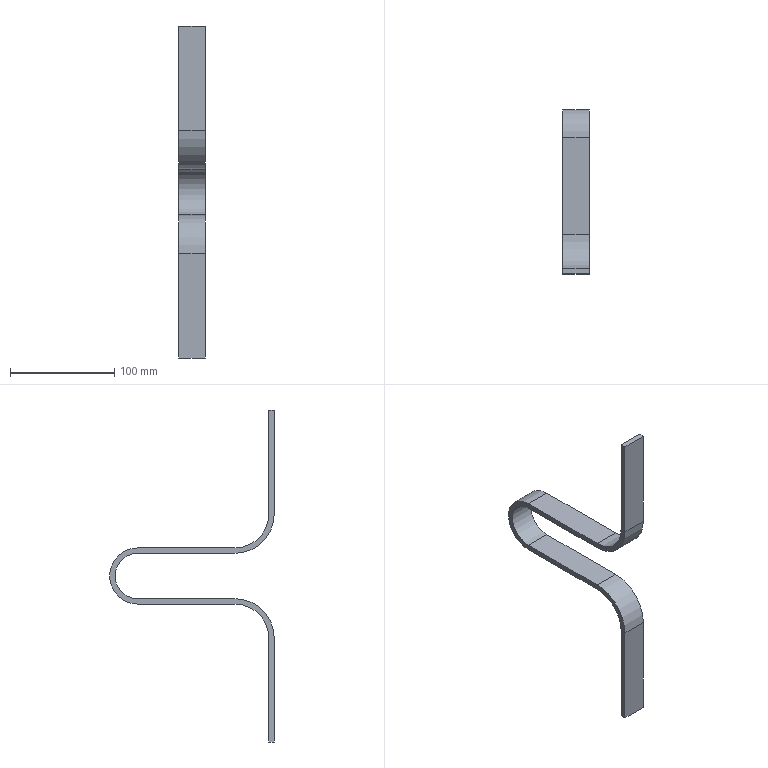Part | STEP file | 0245_Z_103_UM25-8YU-232-SCNUW_2 | 1 solid | 18 faces | box 25 x 158.2 x 319 mm | volume 74610 mm3 | plane 12 | cylinder 6 | commonest cylinder face diameters 65 x2 75.4 x2 43.6 x1 54 x1
STEP:
#1=CARTESIAN_POINT('',(0.,0.,0.));
#2=DIRECTION('',(0.,0.,1.));
#3=DIRECTION('',(1.,0.,0.));
#4=AXIS2_PLACEMENT_3D('',#1,#2,#3);
#5=CARTESIAN_POINT('',(-12.5,5.2,0.));
#6=VERTEX_POINT('',#5);
#7=CARTESIAN_POINT('',(-12.5,0.,0.));
#8=VERTEX_POINT('',#7);
#9=CARTESIAN_POINT('',(-12.5,5.2,0.));
#10=DIRECTION('',(0.,-1.,0.));
#11=VECTOR('',#10,1.);
#12=LINE('',#9,#11);
#13=CARTESIAN_POINT('',(12.5,5.2,0.));
#14=DIRECTION('',(0.,0.,-1.));
#15=DIRECTION('',(-1.,0.,0.));
#16=AXIS2_PLACEMENT_3D('',#13,#14,#15);
#17=PLANE('',#16);
#18=CARTESIAN_POINT('',(25.,0.));
#19=DIRECTION('',(0.,-1.));
#20=VECTOR('',#19,1.);
#21=LINE('',#18,#20);
#22=(GEOMETRIC_REPRESENTATION_CONTEXT(2)PARAMETRIC_REPRESENTATION_CONTEXT()REPRESENTATION_CONTEXT('',''));
#23=DEFINITIONAL_REPRESENTATION('',(#21),#22);
#24=PCURVE('',#17,#23);
#25=CARTESIAN_POINT('',(-12.5,37.7,-100.));
#26=DIRECTION('',(1.,0.,0.));
#27=DIRECTION('',(0.,0.,-1.));
#28=AXIS2_PLACEMENT_3D('',#25,#26,#27);
#29=PLANE('',#28);
#30=CARTESIAN_POINT('',(-100.,-32.5));
#31=DIRECTION('',(0.,-1.));
#32=VECTOR('',#31,1.);
#33=LINE('',#30,#32);
#34=(GEOMETRIC_REPRESENTATION_CONTEXT(2)PARAMETRIC_REPRESENTATION_CONTEXT()REPRESENTATION_CONTEXT('',''));
#35=DEFINITIONAL_REPRESENTATION('',(#33),#34);
#36=PCURVE('',#29,#35);
#37=SURFACE_CURVE('',#12,(#24,#36),.PCURVE_S1.);
#38=EDGE_CURVE('',#6,#8,#37,.T.);
#39=ORIENTED_EDGE('',*,*,#38,.T.);
#40=CARTESIAN_POINT('',(12.5,0.,0.));
#41=VERTEX_POINT('',#40);
#42=CARTESIAN_POINT('',(12.5,0.,0.));
#43=DIRECTION('',(-1.,0.,0.));
#44=VECTOR('',#43,1.);
#45=LINE('',#42,#44);
#46=CARTESIAN_POINT('',(0.,-5.2));
#47=DIRECTION('',(1.,0.));
#48=VECTOR('',#47,1.);
#49=LINE('',#46,#48);
#50=(GEOMETRIC_REPRESENTATION_CONTEXT(2)PARAMETRIC_REPRESENTATION_CONTEXT()REPRESENTATION_CONTEXT('',''));
#51=DEFINITIONAL_REPRESENTATION('',(#49),#50);
#52=PCURVE('',#17,#51);
#53=CARTESIAN_POINT('',(12.5,0.,0.));
#54=DIRECTION('',(0.,1.,0.));
#55=DIRECTION('',(0.,0.,1.));
#56=AXIS2_PLACEMENT_3D('',#53,#54,#55);
#57=PLANE('',#56);
#58=CARTESIAN_POINT('',(0.,0.));
#59=DIRECTION('',(0.,-1.));
#60=VECTOR('',#59,1.);
#61=LINE('',#58,#60);
#62=(GEOMETRIC_REPRESENTATION_CONTEXT(2)PARAMETRIC_REPRESENTATION_CONTEXT()REPRESENTATION_CONTEXT('',''));
#63=DEFINITIONAL_REPRESENTATION('',(#61),#62);
#64=PCURVE('',#57,#63);
#65=SURFACE_CURVE('',#45,(#52,#64),.PCURVE_S1.);
#66=EDGE_CURVE('',#41,#8,#65,.T.);
#67=ORIENTED_EDGE('',*,*,#66,.F.);
#68=CARTESIAN_POINT('',(12.5,5.2,0.));
#69=VERTEX_POINT('',#68);
#70=CARTESIAN_POINT('',(12.5,5.2,0.));
#71=DIRECTION('',(0.,-1.,0.));
#72=VECTOR('',#71,1.);
#73=LINE('',#70,#72);
#74=CARTESIAN_POINT('',(0.,0.));
#75=DIRECTION('',(0.,-1.));
#76=VECTOR('',#75,1.);
#77=LINE('',#74,#76);
#78=(GEOMETRIC_REPRESENTATION_CONTEXT(2)PARAMETRIC_REPRESENTATION_CONTEXT()REPRESENTATION_CONTEXT('',''));
#79=DEFINITIONAL_REPRESENTATION('',(#77),#78);
#80=PCURVE('',#17,#79);
#81=CARTESIAN_POINT('',(12.5,37.7,-100.));
#82=DIRECTION('',(1.,0.,0.));
#83=DIRECTION('',(0.,0.,-1.));
#84=AXIS2_PLACEMENT_3D('',#81,#82,#83);
#85=PLANE('',#84);
#86=CARTESIAN_POINT('',(-100.,-32.5));
#87=DIRECTION('',(0.,-1.));
#88=VECTOR('',#87,1.);
#89=LINE('',#86,#88);
#90=(GEOMETRIC_REPRESENTATION_CONTEXT(2)PARAMETRIC_REPRESENTATION_CONTEXT()REPRESENTATION_CONTEXT('',''));
#91=DEFINITIONAL_REPRESENTATION('',(#89),#90);
#92=PCURVE('',#85,#91);
#93=SURFACE_CURVE('',#73,(#80,#92),.PCURVE_S1.);
#94=EDGE_CURVE('',#69,#41,#93,.T.);
#95=ORIENTED_EDGE('',*,*,#94,.F.);
#96=CARTESIAN_POINT('',(12.5,5.2,0.));
#97=DIRECTION('',(-1.,0.,0.));
#98=VECTOR('',#97,1.);
#99=LINE('',#96,#98);
#100=CARTESIAN_POINT('',(0.,0.));
#101=DIRECTION('',(1.,0.));
#102=VECTOR('',#101,1.);
#103=LINE('',#100,#102);
#104=(GEOMETRIC_REPRESENTATION_CONTEXT(2)PARAMETRIC_REPRESENTATION_CONTEXT()REPRESENTATION_CONTEXT('',''));
#105=DEFINITIONAL_REPRESENTATION('',(#103),#104);
#106=PCURVE('',#17,#105);
#107=CARTESIAN_POINT('',(12.5,5.2,0.));
#108=DIRECTION('',(0.,-1.,0.));
#109=DIRECTION('',(0.,0.,-1.));
#110=AXIS2_PLACEMENT_3D('',#107,#108,#109);
#111=PLANE('',#110);
#112=CARTESIAN_POINT('',(0.,0.));
#113=DIRECTION('',(0.,-1.));
#114=VECTOR('',#113,1.);
#115=LINE('',#112,#114);
#116=(GEOMETRIC_REPRESENTATION_CONTEXT(2)PARAMETRIC_REPRESENTATION_CONTEXT()REPRESENTATION_CONTEXT('',''));
#117=DEFINITIONAL_REPRESENTATION('',(#115),#116);
#118=PCURVE('',#111,#117);
#119=SURFACE_CURVE('',#99,(#106,#118),.PCURVE_S1.);
#120=EDGE_CURVE('',#69,#6,#119,.T.);
#121=ORIENTED_EDGE('',*,*,#120,.T.);
#122=EDGE_LOOP('',(#39,#67,#95,#121));
#123=FACE_BOUND('',#122,.T.);
#124=ADVANCED_FACE('',(#123),#17,.F.);
#125=CARTESIAN_POINT('',(-12.5,0.,-100.));
#126=VERTEX_POINT('',#125);
#127=CARTESIAN_POINT('',(-12.5,0.,0.));
#128=DIRECTION('',(0.,0.,-1.));
#129=VECTOR('',#128,1.);
#130=LINE('',#127,#129);
#131=CARTESIAN_POINT('',(0.,-25.));
#132=DIRECTION('',(-1.,0.));
#133=VECTOR('',#132,1.);
#134=LINE('',#131,#133);
#135=(GEOMETRIC_REPRESENTATION_CONTEXT(2)PARAMETRIC_REPRESENTATION_CONTEXT()REPRESENTATION_CONTEXT('',''));
#136=DEFINITIONAL_REPRESENTATION('',(#134),#135);
#137=PCURVE('',#57,#136);
#138=CARTESIAN_POINT('',(-100.,-37.7));
#139=DIRECTION('',(1.,0.));
#140=VECTOR('',#139,1.);
#141=LINE('',#138,#140);
#142=(GEOMETRIC_REPRESENTATION_CONTEXT(2)PARAMETRIC_REPRESENTATION_CONTEXT()REPRESENTATION_CONTEXT('',''));
#143=DEFINITIONAL_REPRESENTATION('',(#141),#142);
#144=PCURVE('',#29,#143);
#145=SURFACE_CURVE('',#130,(#137,#144),.PCURVE_S1.);
#146=EDGE_CURVE('',#8,#126,#145,.T.);
#147=ORIENTED_EDGE('',*,*,#146,.T.);
#148=CARTESIAN_POINT('',(12.5,0.,-100.));
#149=VERTEX_POINT('',#148);
#150=CARTESIAN_POINT('',(12.5,0.,-100.));
#151=DIRECTION('',(-1.,0.,0.));
#152=VECTOR('',#151,1.);
#153=LINE('',#150,#152);
#154=CARTESIAN_POINT('',(-100.,0.));
#155=DIRECTION('',(0.,-1.));
#156=VECTOR('',#155,1.);
#157=LINE('',#154,#156);
#158=(GEOMETRIC_REPRESENTATION_CONTEXT(2)PARAMETRIC_REPRESENTATION_CONTEXT()REPRESENTATION_CONTEXT('',''));
#159=DEFINITIONAL_REPRESENTATION('',(#157),#158);
#160=PCURVE('',#57,#159);
#161=CARTESIAN_POINT('',(12.5,37.7,-100.));
#162=DIRECTION('',(-1.,0.,0.));
#163=DIRECTION('',(0.,0.,1.));
#164=AXIS2_PLACEMENT_3D('',#161,#162,#163);
#165=CYLINDRICAL_SURFACE('',#164,37.7);
#166=CARTESIAN_POINT('',(4.712,0.));
#167=DIRECTION('',(0.,1.));
#168=VECTOR('',#167,1.);
#169=LINE('',#166,#168);
#170=(GEOMETRIC_REPRESENTATION_CONTEXT(2)PARAMETRIC_REPRESENTATION_CONTEXT()REPRESENTATION_CONTEXT('',''));
#171=DEFINITIONAL_REPRESENTATION('',(#169),#170);
#172=PCURVE('',#165,#171);
#173=SURFACE_CURVE('',#153,(#160,#172),.PCURVE_S1.);
#174=EDGE_CURVE('',#149,#126,#173,.T.);
#175=ORIENTED_EDGE('',*,*,#174,.F.);
#176=CARTESIAN_POINT('',(12.5,0.,0.));
#177=DIRECTION('',(0.,0.,-1.));
#178=VECTOR('',#177,1.);
#179=LINE('',#176,#178);
#180=CARTESIAN_POINT('',(0.,0.));
#181=DIRECTION('',(-1.,0.));
#182=VECTOR('',#181,1.);
#183=LINE('',#180,#182);
#184=(GEOMETRIC_REPRESENTATION_CONTEXT(2)PARAMETRIC_REPRESENTATION_CONTEXT()REPRESENTATION_CONTEXT('',''));
#185=DEFINITIONAL_REPRESENTATION('',(#183),#184);
#186=PCURVE('',#57,#185);
#187=CARTESIAN_POINT('',(-100.,-37.7));
#188=DIRECTION('',(1.,0.));
#189=VECTOR('',#188,1.);
#190=LINE('',#187,#189);
#191=(GEOMETRIC_REPRESENTATION_CONTEXT(2)PARAMETRIC_REPRESENTATION_CONTEXT()REPRESENTATION_CONTEXT('',''));
#192=DEFINITIONAL_REPRESENTATION('',(#190),#191);
#193=PCURVE('',#85,#192);
#194=SURFACE_CURVE('',#179,(#186,#193),.PCURVE_S1.);
#195=EDGE_CURVE('',#41,#149,#194,.T.);
#196=ORIENTED_EDGE('',*,*,#195,.F.);
#197=ORIENTED_EDGE('',*,*,#66,.T.);
#198=EDGE_LOOP('',(#147,#175,#196,#197));
#199=FACE_BOUND('',#198,.T.);
#200=ADVANCED_FACE('',(#199),#57,.F.);
#201=CARTESIAN_POINT('',(-12.5,37.7,-137.7));
#202=VERTEX_POINT('',#201);
#203=CARTESIAN_POINT('',(-12.5,37.7,-100.));
#204=DIRECTION('',(1.,0.,0.));
#205=DIRECTION('',(0.,0.,-1.));
#206=AXIS2_PLACEMENT_3D('',#203,#204,#205);
#207=CIRCLE('',#206,37.7);
#208=CARTESIAN_POINT('',(9.425,25.));
#209=DIRECTION('',(-1.,0.));
#210=VECTOR('',#209,1.);
#211=LINE('',#208,#210);
#212=(GEOMETRIC_REPRESENTATION_CONTEXT(2)PARAMETRIC_REPRESENTATION_CONTEXT()REPRESENTATION_CONTEXT('',''));
#213=DEFINITIONAL_REPRESENTATION('',(#211),#212);
#214=PCURVE('',#165,#213);
#215=CARTESIAN_POINT('',(0.,0.));
#216=DIRECTION('',(1.,0.));
#217=AXIS2_PLACEMENT_2D('',#215,#216);
#218=CIRCLE('',#217,37.7);
#219=(GEOMETRIC_REPRESENTATION_CONTEXT(2)PARAMETRIC_REPRESENTATION_CONTEXT()REPRESENTATION_CONTEXT('',''));
#220=DEFINITIONAL_REPRESENTATION('',(#218),#219);
#221=PCURVE('',#29,#220);
#222=SURFACE_CURVE('',#207,(#214,#221),.PCURVE_S1.);
#223=EDGE_CURVE('',#126,#202,#222,.T.);
#224=ORIENTED_EDGE('',*,*,#223,.T.);
#225=CARTESIAN_POINT('',(12.5,37.7,-137.7));
#226=VERTEX_POINT('',#225);
#227=CARTESIAN_POINT('',(12.5,37.7,-137.7));
#228=DIRECTION('',(-1.,0.,0.));
#229=VECTOR('',#228,1.);
#230=LINE('',#227,#229);
#231=CARTESIAN_POINT('',(3.142,0.));
#232=DIRECTION('',(0.,1.));
#233=VECTOR('',#232,1.);
#234=LINE('',#231,#233);
#235=(GEOMETRIC_REPRESENTATION_CONTEXT(2)PARAMETRIC_REPRESENTATION_CONTEXT()REPRESENTATION_CONTEXT('',''));
#236=DEFINITIONAL_REPRESENTATION('',(#234),#235);
#237=PCURVE('',#165,#236);
#238=CARTESIAN_POINT('',(12.5,37.7,-137.7));
#239=DIRECTION('',(0.,0.,1.));
#240=DIRECTION('',(0.,-1.,0.));
#241=AXIS2_PLACEMENT_3D('',#238,#239,#240);
#242=PLANE('',#241);
#243=CARTESIAN_POINT('',(0.,0.));
#244=DIRECTION('',(0.,-1.));
#245=VECTOR('',#244,1.);
#246=LINE('',#243,#245);
#247=(GEOMETRIC_REPRESENTATION_CONTEXT(2)PARAMETRIC_REPRESENTATION_CONTEXT()REPRESENTATION_CONTEXT('',''));
#248=DEFINITIONAL_REPRESENTATION('',(#246),#247);
#249=PCURVE('',#242,#248);
#250=SURFACE_CURVE('',#230,(#237,#249),.PCURVE_S1.);
#251=EDGE_CURVE('',#226,#202,#250,.T.);
#252=ORIENTED_EDGE('',*,*,#251,.F.);
#253=CARTESIAN_POINT('',(12.5,37.7,-100.));
#254=DIRECTION('',(1.,0.,0.));
#255=DIRECTION('',(0.,0.,-1.));
#256=AXIS2_PLACEMENT_3D('',#253,#254,#255);
#257=CIRCLE('',#256,37.7);
#258=CARTESIAN_POINT('',(9.425,0.));
#259=DIRECTION('',(-1.,0.));
#260=VECTOR('',#259,1.);
#261=LINE('',#258,#260);
#262=(GEOMETRIC_REPRESENTATION_CONTEXT(2)PARAMETRIC_REPRESENTATION_CONTEXT()REPRESENTATION_CONTEXT('',''));
#263=DEFINITIONAL_REPRESENTATION('',(#261),#262);
#264=PCURVE('',#165,#263);
#265=CARTESIAN_POINT('',(0.,0.));
#266=DIRECTION('',(1.,0.));
#267=AXIS2_PLACEMENT_2D('',#265,#266);
#268=CIRCLE('',#267,37.7);
#269=(GEOMETRIC_REPRESENTATION_CONTEXT(2)PARAMETRIC_REPRESENTATION_CONTEXT()REPRESENTATION_CONTEXT('',''));
#270=DEFINITIONAL_REPRESENTATION('',(#268),#269);
#271=PCURVE('',#85,#270);
#272=SURFACE_CURVE('',#257,(#264,#271),.PCURVE_S1.);
#273=EDGE_CURVE('',#149,#226,#272,.T.);
#274=ORIENTED_EDGE('',*,*,#273,.F.);
#275=ORIENTED_EDGE('',*,*,#174,.T.);
#276=EDGE_LOOP('',(#224,#252,#274,#275));
#277=FACE_BOUND('',#276,.T.);
#278=ADVANCED_FACE('',(#277),#165,.T.);
#279=CARTESIAN_POINT('',(-12.5,131.2,-137.7));
#280=VERTEX_POINT('',#279);
#281=CARTESIAN_POINT('',(-12.5,37.7,-137.7));
#282=DIRECTION('',(0.,1.,0.));
#283=VECTOR('',#282,1.);
#284=LINE('',#281,#283);
#285=CARTESIAN_POINT('',(0.,-25.));
#286=DIRECTION('',(-1.,0.));
#287=VECTOR('',#286,1.);
#288=LINE('',#285,#287);
#289=(GEOMETRIC_REPRESENTATION_CONTEXT(2)PARAMETRIC_REPRESENTATION_CONTEXT()REPRESENTATION_CONTEXT('',''));
#290=DEFINITIONAL_REPRESENTATION('',(#288),#289);
#291=PCURVE('',#242,#290);
#292=CARTESIAN_POINT('',(37.7,0.));
#293=DIRECTION('',(0.,1.));
#294=VECTOR('',#293,1.);
#295=LINE('',#292,#294);
#296=(GEOMETRIC_REPRESENTATION_CONTEXT(2)PARAMETRIC_REPRESENTATION_CONTEXT()REPRESENTATION_CONTEXT('',''));
#297=DEFINITIONAL_REPRESENTATION('',(#295),#296);
#298=PCURVE('',#29,#297);
#299=SURFACE_CURVE('',#284,(#291,#298),.PCURVE_S1.);
#300=EDGE_CURVE('',#202,#280,#299,.T.);
#301=ORIENTED_EDGE('',*,*,#300,.T.);
#302=CARTESIAN_POINT('',(12.5,131.2,-137.7));
#303=VERTEX_POINT('',#302);
#304=CARTESIAN_POINT('',(12.5,131.2,-137.7));
#305=DIRECTION('',(-1.,0.,0.));
#306=VECTOR('',#305,1.);
#307=LINE('',#304,#306);
#308=CARTESIAN_POINT('',(-93.5,0.));
#309=DIRECTION('',(0.,-1.));
#310=VECTOR('',#309,1.);
#311=LINE('',#308,#310);
#312=(GEOMETRIC_REPRESENTATION_CONTEXT(2)PARAMETRIC_REPRESENTATION_CONTEXT()REPRESENTATION_CONTEXT('',''));
#313=DEFINITIONAL_REPRESENTATION('',(#311),#312);
#314=PCURVE('',#242,#313);
#315=CARTESIAN_POINT('',(12.5,131.2,-159.5));
#316=DIRECTION('',(-1.,0.,0.));
#317=DIRECTION('',(0.,0.,1.));
#318=AXIS2_PLACEMENT_3D('',#315,#316,#317);
#319=CYLINDRICAL_SURFACE('',#318,21.8);
#320=CARTESIAN_POINT('',(0.,0.));
#321=DIRECTION('',(0.,1.));
#322=VECTOR('',#321,1.);
#323=LINE('',#320,#322);
#324=(GEOMETRIC_REPRESENTATION_CONTEXT(2)PARAMETRIC_REPRESENTATION_CONTEXT()REPRESENTATION_CONTEXT('',''));
#325=DEFINITIONAL_REPRESENTATION('',(#323),#324);
#326=PCURVE('',#319,#325);
#327=SURFACE_CURVE('',#307,(#314,#326),.PCURVE_S1.);
#328=EDGE_CURVE('',#303,#280,#327,.T.);
#329=ORIENTED_EDGE('',*,*,#328,.F.);
#330=CARTESIAN_POINT('',(12.5,37.7,-137.7));
#331=DIRECTION('',(0.,1.,0.));
#332=VECTOR('',#331,1.);
#333=LINE('',#330,#332);
#334=CARTESIAN_POINT('',(0.,0.));
#335=DIRECTION('',(-1.,0.));
#336=VECTOR('',#335,1.);
#337=LINE('',#334,#336);
#338=(GEOMETRIC_REPRESENTATION_CONTEXT(2)PARAMETRIC_REPRESENTATION_CONTEXT()REPRESENTATION_CONTEXT('',''));
#339=DEFINITIONAL_REPRESENTATION('',(#337),#338);
#340=PCURVE('',#242,#339);
#341=CARTESIAN_POINT('',(37.7,0.));
#342=DIRECTION('',(0.,1.));
#343=VECTOR('',#342,1.);
#344=LINE('',#341,#343);
#345=(GEOMETRIC_REPRESENTATION_CONTEXT(2)PARAMETRIC_REPRESENTATION_CONTEXT()REPRESENTATION_CONTEXT('',''));
#346=DEFINITIONAL_REPRESENTATION('',(#344),#345);
#347=PCURVE('',#85,#346);
#348=SURFACE_CURVE('',#333,(#340,#347),.PCURVE_S1.);
#349=EDGE_CURVE('',#226,#303,#348,.T.);
#350=ORIENTED_EDGE('',*,*,#349,.F.);
#351=ORIENTED_EDGE('',*,*,#251,.T.);
#352=EDGE_LOOP('',(#301,#329,#350,#351));
#353=FACE_BOUND('',#352,.T.);
#354=ADVANCED_FACE('',(#353),#242,.F.);
#355=ORIENTED_EDGE('',*,*,#328,.F.);
#356=CARTESIAN_POINT('',(12.5,131.2,-181.3));
#357=VERTEX_POINT('',#356);
#358=CARTESIAN_POINT('',(12.5,131.2,-159.5));
#359=DIRECTION('',(-1.,0.,0.));
#360=DIRECTION('',(0.,0.,1.));
#361=AXIS2_PLACEMENT_3D('',#358,#359,#360);
#362=CIRCLE('',#361,21.8);
#363=CARTESIAN_POINT('',(0.,0.));
#364=DIRECTION('',(1.,0.));
#365=VECTOR('',#364,1.);
#366=LINE('',#363,#365);
#367=(GEOMETRIC_REPRESENTATION_CONTEXT(2)PARAMETRIC_REPRESENTATION_CONTEXT()REPRESENTATION_CONTEXT('',''));
#368=DEFINITIONAL_REPRESENTATION('',(#366),#367);
#369=PCURVE('',#319,#368);
#370=CARTESIAN_POINT('',(37.7,93.5));
#371=CARTESIAN_POINT('',(37.7,131.259));
#372=CARTESIAN_POINT('',(70.4,112.379));
#373=CARTESIAN_POINT('',(103.1,93.5));
#374=CARTESIAN_POINT('',(70.4,74.621));
#375=CARTESIAN_POINT('',(37.7,55.741));
#376=CARTESIAN_POINT('',(37.7,93.5));
#377=(BOUNDED_CURVE()B_SPLINE_CURVE(2,(#370,#371,#372,#373,#374,#375,#376),.UNSPECIFIED.,.T.,.F.)B_SPLINE_CURVE_WITH_KNOTS((1,2,2,2,2,1),(-2.094,0.,2.094,4.189,6.283,8.378),.UNSPECIFIED.)CURVE()GEOMETRIC_REPRESENTATION_ITEM()RATIONAL_B_SPLINE_CURVE((1.,0.5,1.,0.5,1.,0.5,1.))REPRESENTATION_ITEM(''));
#378=(GEOMETRIC_REPRESENTATION_CONTEXT(2)PARAMETRIC_REPRESENTATION_CONTEXT()REPRESENTATION_CONTEXT('',''));
#379=DEFINITIONAL_REPRESENTATION('',(#377),#378);
#380=PCURVE('',#85,#379);
#381=SURFACE_CURVE('',#362,(#369,#380),.PCURVE_S1.);
#382=EDGE_CURVE('',#303,#357,#381,.T.);
#383=ORIENTED_EDGE('',*,*,#382,.T.);
#384=CARTESIAN_POINT('',(-12.5,131.2,-181.3));
#385=VERTEX_POINT('',#384);
#386=CARTESIAN_POINT('',(12.5,131.2,-181.3));
#387=DIRECTION('',(-1.,0.,0.));
#388=VECTOR('',#387,1.);
#389=LINE('',#386,#388);
#390=CARTESIAN_POINT('',(3.142,0.));
#391=DIRECTION('',(0.,1.));
#392=VECTOR('',#391,1.);
#393=LINE('',#390,#392);
#394=(GEOMETRIC_REPRESENTATION_CONTEXT(2)PARAMETRIC_REPRESENTATION_CONTEXT()REPRESENTATION_CONTEXT('',''));
#395=DEFINITIONAL_REPRESENTATION('',(#393),#394);
#396=PCURVE('',#319,#395);
#397=CARTESIAN_POINT('',(12.5,131.2,-181.3));
#398=DIRECTION('',(0.,0.,-1.));
#399=DIRECTION('',(0.,1.,0.));
#400=AXIS2_PLACEMENT_3D('',#397,#398,#399);
#401=PLANE('',#400);
#402=CARTESIAN_POINT('',(0.,0.));
#403=DIRECTION('',(0.,-1.));
#404=VECTOR('',#403,1.);
#405=LINE('',#402,#404);
#406=(GEOMETRIC_REPRESENTATION_CONTEXT(2)PARAMETRIC_REPRESENTATION_CONTEXT()REPRESENTATION_CONTEXT('',''));
#407=DEFINITIONAL_REPRESENTATION('',(#405),#406);
#408=PCURVE('',#401,#407);
#409=SURFACE_CURVE('',#389,(#396,#408),.PCURVE_S1.);
#410=EDGE_CURVE('',#357,#385,#409,.T.);
#411=ORIENTED_EDGE('',*,*,#410,.T.);
#412=CARTESIAN_POINT('',(-12.5,131.2,-159.5));
#413=DIRECTION('',(-1.,0.,0.));
#414=DIRECTION('',(0.,0.,1.));
#415=AXIS2_PLACEMENT_3D('',#412,#413,#414);
#416=CIRCLE('',#415,21.8);
#417=CARTESIAN_POINT('',(0.,25.));
#418=DIRECTION('',(1.,0.));
#419=VECTOR('',#418,1.);
#420=LINE('',#417,#419);
#421=(GEOMETRIC_REPRESENTATION_CONTEXT(2)PARAMETRIC_REPRESENTATION_CONTEXT()REPRESENTATION_CONTEXT('',''));
#422=DEFINITIONAL_REPRESENTATION('',(#420),#421);
#423=PCURVE('',#319,#422);
#424=CARTESIAN_POINT('',(37.7,93.5));
#425=CARTESIAN_POINT('',(37.7,131.259));
#426=CARTESIAN_POINT('',(70.4,112.379));
#427=CARTESIAN_POINT('',(103.1,93.5));
#428=CARTESIAN_POINT('',(70.4,74.621));
#429=CARTESIAN_POINT('',(37.7,55.741));
#430=CARTESIAN_POINT('',(37.7,93.5));
#431=(BOUNDED_CURVE()B_SPLINE_CURVE(2,(#424,#425,#426,#427,#428,#429,#430),.UNSPECIFIED.,.T.,.F.)B_SPLINE_CURVE_WITH_KNOTS((1,2,2,2,2,1),(-2.094,0.,2.094,4.189,6.283,8.378),.UNSPECIFIED.)CURVE()GEOMETRIC_REPRESENTATION_ITEM()RATIONAL_B_SPLINE_CURVE((1.,0.5,1.,0.5,1.,0.5,1.))REPRESENTATION_ITEM(''));
#432=(GEOMETRIC_REPRESENTATION_CONTEXT(2)PARAMETRIC_REPRESENTATION_CONTEXT()REPRESENTATION_CONTEXT('',''));
#433=DEFINITIONAL_REPRESENTATION('',(#431),#432);
#434=PCURVE('',#29,#433);
#435=SURFACE_CURVE('',#416,(#423,#434),.PCURVE_S1.);
#436=EDGE_CURVE('',#280,#385,#435,.T.);
#437=ORIENTED_EDGE('',*,*,#436,.F.);
#438=EDGE_LOOP('',(#355,#383,#411,#437));
#439=FACE_BOUND('',#438,.F.);
#440=ADVANCED_FACE('',(#439),#319,.F.);
#441=CARTESIAN_POINT('',(-12.5,37.7,-181.3));
#442=VERTEX_POINT('',#441);
#443=CARTESIAN_POINT('',(-12.5,131.2,-181.3));
#444=DIRECTION('',(0.,-1.,0.));
#445=VECTOR('',#444,1.);
#446=LINE('',#443,#445);
#447=CARTESIAN_POINT('',(0.,-25.));
#448=DIRECTION('',(-1.,0.));
#449=VECTOR('',#448,1.);
#450=LINE('',#447,#449);
#451=(GEOMETRIC_REPRESENTATION_CONTEXT(2)PARAMETRIC_REPRESENTATION_CONTEXT()REPRESENTATION_CONTEXT('',''));
#452=DEFINITIONAL_REPRESENTATION('',(#450),#451);
#453=PCURVE('',#401,#452);
#454=CARTESIAN_POINT('',(81.3,93.5));
#455=DIRECTION('',(0.,-1.));
#456=VECTOR('',#455,1.);
#457=LINE('',#454,#456);
#458=(GEOMETRIC_REPRESENTATION_CONTEXT(2)PARAMETRIC_REPRESENTATION_CONTEXT()REPRESENTATION_CONTEXT('',''));
#459=DEFINITIONAL_REPRESENTATION('',(#457),#458);
#460=PCURVE('',#29,#459);
#461=SURFACE_CURVE('',#446,(#453,#460),.PCURVE_S1.);
#462=EDGE_CURVE('',#385,#442,#461,.T.);
#463=ORIENTED_EDGE('',*,*,#462,.T.);
#464=CARTESIAN_POINT('',(12.5,37.7,-181.3));
#465=VERTEX_POINT('',#464);
#466=CARTESIAN_POINT('',(12.5,37.7,-181.3));
#467=DIRECTION('',(-1.,0.,0.));
#468=VECTOR('',#467,1.);
#469=LINE('',#466,#468);
#470=CARTESIAN_POINT('',(-93.5,0.));
#471=DIRECTION('',(0.,-1.));
#472=VECTOR('',#471,1.);
#473=LINE('',#470,#472);
#474=(GEOMETRIC_REPRESENTATION_CONTEXT(2)PARAMETRIC_REPRESENTATION_CONTEXT()REPRESENTATION_CONTEXT('',''));
#475=DEFINITIONAL_REPRESENTATION('',(#473),#474);
#476=PCURVE('',#401,#475);
#477=CARTESIAN_POINT('',(12.5,37.7,-219.));
#478=DIRECTION('',(-1.,0.,0.));
#479=DIRECTION('',(0.,0.,1.));
#480=AXIS2_PLACEMENT_3D('',#477,#478,#479);
#481=CYLINDRICAL_SURFACE('',#480,37.7);
#482=CARTESIAN_POINT('',(6.283,0.));
#483=DIRECTION('',(0.,1.));
#484=VECTOR('',#483,1.);
#485=LINE('',#482,#484);
#486=(GEOMETRIC_REPRESENTATION_CONTEXT(2)PARAMETRIC_REPRESENTATION_CONTEXT()REPRESENTATION_CONTEXT('',''));
#487=DEFINITIONAL_REPRESENTATION('',(#485),#486);
#488=PCURVE('',#481,#487);
#489=SURFACE_CURVE('',#469,(#476,#488),.PCURVE_S1.);
#490=EDGE_CURVE('',#465,#442,#489,.T.);
#491=ORIENTED_EDGE('',*,*,#490,.F.);
#492=CARTESIAN_POINT('',(12.5,131.2,-181.3));
#493=DIRECTION('',(0.,-1.,0.));
#494=VECTOR('',#493,1.);
#495=LINE('',#492,#494);
#496=CARTESIAN_POINT('',(0.,0.));
#497=DIRECTION('',(-1.,0.));
#498=VECTOR('',#497,1.);
#499=LINE('',#496,#498);
#500=(GEOMETRIC_REPRESENTATION_CONTEXT(2)PARAMETRIC_REPRESENTATION_CONTEXT()REPRESENTATION_CONTEXT('',''));
#501=DEFINITIONAL_REPRESENTATION('',(#499),#500);
#502=PCURVE('',#401,#501);
#503=CARTESIAN_POINT('',(81.3,93.5));
#504=DIRECTION('',(0.,-1.));
#505=VECTOR('',#504,1.);
#506=LINE('',#503,#505);
#507=(GEOMETRIC_REPRESENTATION_CONTEXT(2)PARAMETRIC_REPRESENTATION_CONTEXT()REPRESENTATION_CONTEXT('',''));
#508=DEFINITIONAL_REPRESENTATION('',(#506),#507);
#509=PCURVE('',#85,#508);
#510=SURFACE_CURVE('',#495,(#502,#509),.PCURVE_S1.);
#511=EDGE_CURVE('',#357,#465,#510,.T.);
#512=ORIENTED_EDGE('',*,*,#511,.F.);
#513=ORIENTED_EDGE('',*,*,#410,.T.);
#514=EDGE_LOOP('',(#463,#491,#512,#513));
#515=FACE_BOUND('',#514,.T.);
#516=ADVANCED_FACE('',(#515),#401,.F.);
#517=CARTESIAN_POINT('',(-12.5,0.,-219.));
#518=VERTEX_POINT('',#517);
#519=CARTESIAN_POINT('',(-12.5,37.7,-219.));
#520=DIRECTION('',(1.,0.,0.));
#521=DIRECTION('',(0.,0.,-1.));
#522=AXIS2_PLACEMENT_3D('',#519,#520,#521);
#523=CIRCLE('',#522,37.7);
#524=CARTESIAN_POINT('',(9.425,25.));
#525=DIRECTION('',(-1.,0.));
#526=VECTOR('',#525,1.);
#527=LINE('',#524,#526);
#528=(GEOMETRIC_REPRESENTATION_CONTEXT(2)PARAMETRIC_REPRESENTATION_CONTEXT()REPRESENTATION_CONTEXT('',''));
#529=DEFINITIONAL_REPRESENTATION('',(#527),#528);
#530=PCURVE('',#481,#529);
#531=CARTESIAN_POINT('',(119.,0.));
#532=DIRECTION('',(1.,0.));
#533=AXIS2_PLACEMENT_2D('',#531,#532);
#534=CIRCLE('',#533,37.7);
#535=(GEOMETRIC_REPRESENTATION_CONTEXT(2)PARAMETRIC_REPRESENTATION_CONTEXT()REPRESENTATION_CONTEXT('',''));
#536=DEFINITIONAL_REPRESENTATION('',(#534),#535);
#537=PCURVE('',#29,#536);
#538=SURFACE_CURVE('',#523,(#530,#537),.PCURVE_S1.);
#539=EDGE_CURVE('',#442,#518,#538,.T.);
#540=ORIENTED_EDGE('',*,*,#539,.T.);
#541=CARTESIAN_POINT('',(12.5,0.,-219.));
#542=VERTEX_POINT('',#541);
#543=CARTESIAN_POINT('',(12.5,0.,-219.));
#544=DIRECTION('',(-1.,0.,0.));
#545=VECTOR('',#544,1.);
#546=LINE('',#543,#545);
#547=CARTESIAN_POINT('',(4.712,0.));
#548=DIRECTION('',(0.,1.));
#549=VECTOR('',#548,1.);
#550=LINE('',#547,#549);
#551=(GEOMETRIC_REPRESENTATION_CONTEXT(2)PARAMETRIC_REPRESENTATION_CONTEXT()REPRESENTATION_CONTEXT('',''));
#552=DEFINITIONAL_REPRESENTATION('',(#550),#551);
#553=PCURVE('',#481,#552);
#554=CARTESIAN_POINT('',(12.5,0.,-219.));
#555=DIRECTION('',(0.,1.,0.));
#556=DIRECTION('',(0.,0.,1.));
#557=AXIS2_PLACEMENT_3D('',#554,#555,#556);
#558=PLANE('',#557);
#559=CARTESIAN_POINT('',(0.,0.));
#560=DIRECTION('',(0.,-1.));
#561=VECTOR('',#560,1.);
#562=LINE('',#559,#561);
#563=(GEOMETRIC_REPRESENTATION_CONTEXT(2)PARAMETRIC_REPRESENTATION_CONTEXT()REPRESENTATION_CONTEXT('',''));
#564=DEFINITIONAL_REPRESENTATION('',(#562),#563);
#565=PCURVE('',#558,#564);
#566=SURFACE_CURVE('',#546,(#553,#565),.PCURVE_S1.);
#567=EDGE_CURVE('',#542,#518,#566,.T.);
#568=ORIENTED_EDGE('',*,*,#567,.F.);
#569=CARTESIAN_POINT('',(12.5,37.7,-219.));
#570=DIRECTION('',(1.,0.,0.));
#571=DIRECTION('',(0.,0.,-1.));
#572=AXIS2_PLACEMENT_3D('',#569,#570,#571);
#573=CIRCLE('',#572,37.7);
#574=CARTESIAN_POINT('',(9.425,0.));
#575=DIRECTION('',(-1.,0.));
#576=VECTOR('',#575,1.);
#577=LINE('',#574,#576);
#578=(GEOMETRIC_REPRESENTATION_CONTEXT(2)PARAMETRIC_REPRESENTATION_CONTEXT()REPRESENTATION_CONTEXT('',''));
#579=DEFINITIONAL_REPRESENTATION('',(#577),#578);
#580=PCURVE('',#481,#579);
#581=CARTESIAN_POINT('',(119.,0.));
#582=DIRECTION('',(1.,0.));
#583=AXIS2_PLACEMENT_2D('',#581,#582);
#584=CIRCLE('',#583,37.7);
#585=(GEOMETRIC_REPRESENTATION_CONTEXT(2)PARAMETRIC_REPRESENTATION_CONTEXT()REPRESENTATION_CONTEXT('',''));
#586=DEFINITIONAL_REPRESENTATION('',(#584),#585);
#587=PCURVE('',#85,#586);
#588=SURFACE_CURVE('',#573,(#580,#587),.PCURVE_S1.);
#589=EDGE_CURVE('',#465,#542,#588,.T.);
#590=ORIENTED_EDGE('',*,*,#589,.F.);
#591=ORIENTED_EDGE('',*,*,#490,.T.);
#592=EDGE_LOOP('',(#540,#568,#590,#591));
#593=FACE_BOUND('',#592,.T.);
#594=ADVANCED_FACE('',(#593),#481,.T.);
#595=CARTESIAN_POINT('',(-12.5,0.,-319.));
#596=VERTEX_POINT('',#595);
#597=CARTESIAN_POINT('',(-12.5,0.,-219.));
#598=DIRECTION('',(0.,0.,-1.));
#599=VECTOR('',#598,1.);
#600=LINE('',#597,#599);
#601=CARTESIAN_POINT('',(0.,-25.));
#602=DIRECTION('',(-1.,0.));
#603=VECTOR('',#602,1.);
#604=LINE('',#601,#603);
#605=(GEOMETRIC_REPRESENTATION_CONTEXT(2)PARAMETRIC_REPRESENTATION_CONTEXT()REPRESENTATION_CONTEXT('',''));
#606=DEFINITIONAL_REPRESENTATION('',(#604),#605);
#607=PCURVE('',#558,#606);
#608=CARTESIAN_POINT('',(119.,-37.7));
#609=DIRECTION('',(1.,0.));
#610=VECTOR('',#609,1.);
#611=LINE('',#608,#610);
#612=(GEOMETRIC_REPRESENTATION_CONTEXT(2)PARAMETRIC_REPRESENTATION_CONTEXT()REPRESENTATION_CONTEXT('',''));
#613=DEFINITIONAL_REPRESENTATION('',(#611),#612);
#614=PCURVE('',#29,#613);
#615=SURFACE_CURVE('',#600,(#607,#614),.PCURVE_S1.);
#616=EDGE_CURVE('',#518,#596,#615,.T.);
#617=ORIENTED_EDGE('',*,*,#616,.T.);
#618=CARTESIAN_POINT('',(12.5,0.,-319.));
#619=VERTEX_POINT('',#618);
#620=CARTESIAN_POINT('',(12.5,0.,-319.));
#621=DIRECTION('',(-1.,0.,0.));
#622=VECTOR('',#621,1.);
#623=LINE('',#620,#622);
#624=CARTESIAN_POINT('',(-100.,0.));
#625=DIRECTION('',(0.,-1.));
#626=VECTOR('',#625,1.);
#627=LINE('',#624,#626);
#628=(GEOMETRIC_REPRESENTATION_CONTEXT(2)PARAMETRIC_REPRESENTATION_CONTEXT()REPRESENTATION_CONTEXT('',''));
#629=DEFINITIONAL_REPRESENTATION('',(#627),#628);
#630=PCURVE('',#558,#629);
#631=CARTESIAN_POINT('',(12.5,0.,-319.));
#632=DIRECTION('',(0.,0.,1.));
#633=DIRECTION('',(1.,0.,0.));
#634=AXIS2_PLACEMENT_3D('',#631,#632,#633);
#635=PLANE('',#634);
#636=CARTESIAN_POINT('',(0.,0.));
#637=DIRECTION('',(-1.,0.));
#638=VECTOR('',#637,1.);
#639=LINE('',#636,#638);
#640=(GEOMETRIC_REPRESENTATION_CONTEXT(2)PARAMETRIC_REPRESENTATION_CONTEXT()REPRESENTATION_CONTEXT('',''));
#641=DEFINITIONAL_REPRESENTATION('',(#639),#640);
#642=PCURVE('',#635,#641);
#643=SURFACE_CURVE('',#623,(#630,#642),.PCURVE_S1.);
#644=EDGE_CURVE('',#619,#596,#643,.T.);
#645=ORIENTED_EDGE('',*,*,#644,.F.);
#646=CARTESIAN_POINT('',(12.5,0.,-219.));
#647=DIRECTION('',(0.,0.,-1.));
#648=VECTOR('',#647,1.);
#649=LINE('',#646,#648);
#650=CARTESIAN_POINT('',(0.,0.));
#651=DIRECTION('',(-1.,0.));
#652=VECTOR('',#651,1.);
#653=LINE('',#650,#652);
#654=(GEOMETRIC_REPRESENTATION_CONTEXT(2)PARAMETRIC_REPRESENTATION_CONTEXT()REPRESENTATION_CONTEXT('',''));
#655=DEFINITIONAL_REPRESENTATION('',(#653),#654);
#656=PCURVE('',#558,#655);
#657=CARTESIAN_POINT('',(119.,-37.7));
#658=DIRECTION('',(1.,0.));
#659=VECTOR('',#658,1.);
#660=LINE('',#657,#659);
#661=(GEOMETRIC_REPRESENTATION_CONTEXT(2)PARAMETRIC_REPRESENTATION_CONTEXT()REPRESENTATION_CONTEXT('',''));
#662=DEFINITIONAL_REPRESENTATION('',(#660),#661);
#663=PCURVE('',#85,#662);
#664=SURFACE_CURVE('',#649,(#656,#663),.PCURVE_S1.);
#665=EDGE_CURVE('',#542,#619,#664,.T.);
#666=ORIENTED_EDGE('',*,*,#665,.F.);
#667=ORIENTED_EDGE('',*,*,#567,.T.);
#668=EDGE_LOOP('',(#617,#645,#666,#667));
#669=FACE_BOUND('',#668,.T.);
#670=ADVANCED_FACE('',(#669),#558,.F.);
#671=CARTESIAN_POINT('',(-12.5,5.2,-319.));
#672=VERTEX_POINT('',#671);
#673=CARTESIAN_POINT('',(-12.5,0.,-319.));
#674=DIRECTION('',(0.,1.,0.));
#675=VECTOR('',#674,1.);
#676=LINE('',#673,#675);
#677=CARTESIAN_POINT('',(-25.,0.));
#678=DIRECTION('',(0.,1.));
#679=VECTOR('',#678,1.);
#680=LINE('',#677,#679);
#681=(GEOMETRIC_REPRESENTATION_CONTEXT(2)PARAMETRIC_REPRESENTATION_CONTEXT()REPRESENTATION_CONTEXT('',''));
#682=DEFINITIONAL_REPRESENTATION('',(#680),#681);
#683=PCURVE('',#635,#682);
#684=CARTESIAN_POINT('',(219.,-37.7));
#685=DIRECTION('',(0.,1.));
#686=VECTOR('',#685,1.);
#687=LINE('',#684,#686);
#688=(GEOMETRIC_REPRESENTATION_CONTEXT(2)PARAMETRIC_REPRESENTATION_CONTEXT()REPRESENTATION_CONTEXT('',''));
#689=DEFINITIONAL_REPRESENTATION('',(#687),#688);
#690=PCURVE('',#29,#689);
#691=SURFACE_CURVE('',#676,(#683,#690),.PCURVE_S1.);
#692=EDGE_CURVE('',#596,#672,#691,.T.);
#693=ORIENTED_EDGE('',*,*,#692,.T.);
#694=CARTESIAN_POINT('',(12.5,5.2,-319.));
#695=VERTEX_POINT('',#694);
#696=CARTESIAN_POINT('',(12.5,5.2,-319.));
#697=DIRECTION('',(-1.,0.,0.));
#698=VECTOR('',#697,1.);
#699=LINE('',#696,#698);
#700=CARTESIAN_POINT('',(0.,5.2));
#701=DIRECTION('',(-1.,0.));
#702=VECTOR('',#701,1.);
#703=LINE('',#700,#702);
#704=(GEOMETRIC_REPRESENTATION_CONTEXT(2)PARAMETRIC_REPRESENTATION_CONTEXT()REPRESENTATION_CONTEXT('',''));
#705=DEFINITIONAL_REPRESENTATION('',(#703),#704);
#706=PCURVE('',#635,#705);
#707=CARTESIAN_POINT('',(12.5,5.2,-219.));
#708=DIRECTION('',(0.,-1.,0.));
#709=DIRECTION('',(0.,0.,-1.));
#710=AXIS2_PLACEMENT_3D('',#707,#708,#709);
#711=PLANE('',#710);
#712=CARTESIAN_POINT('',(100.,0.));
#713=DIRECTION('',(0.,-1.));
#714=VECTOR('',#713,1.);
#715=LINE('',#712,#714);
#716=(GEOMETRIC_REPRESENTATION_CONTEXT(2)PARAMETRIC_REPRESENTATION_CONTEXT()REPRESENTATION_CONTEXT('',''));
#717=DEFINITIONAL_REPRESENTATION('',(#715),#716);
#718=PCURVE('',#711,#717);
#719=SURFACE_CURVE('',#699,(#706,#718),.PCURVE_S1.);
#720=EDGE_CURVE('',#695,#672,#719,.T.);
#721=ORIENTED_EDGE('',*,*,#720,.F.);
#722=CARTESIAN_POINT('',(12.5,0.,-319.));
#723=DIRECTION('',(0.,1.,0.));
#724=VECTOR('',#723,1.);
#725=LINE('',#722,#724);
#726=CARTESIAN_POINT('',(0.,0.));
#727=DIRECTION('',(0.,1.));
#728=VECTOR('',#727,1.);
#729=LINE('',#726,#728);
#730=(GEOMETRIC_REPRESENTATION_CONTEXT(2)PARAMETRIC_REPRESENTATION_CONTEXT()REPRESENTATION_CONTEXT('',''));
#731=DEFINITIONAL_REPRESENTATION('',(#729),#730);
#732=PCURVE('',#635,#731);
#733=CARTESIAN_POINT('',(219.,-37.7));
#734=DIRECTION('',(0.,1.));
#735=VECTOR('',#734,1.);
#736=LINE('',#733,#735);
#737=(GEOMETRIC_REPRESENTATION_CONTEXT(2)PARAMETRIC_REPRESENTATION_CONTEXT()REPRESENTATION_CONTEXT('',''));
#738=DEFINITIONAL_REPRESENTATION('',(#736),#737);
#739=PCURVE('',#85,#738);
#740=SURFACE_CURVE('',#725,(#732,#739),.PCURVE_S1.);
#741=EDGE_CURVE('',#619,#695,#740,.T.);
#742=ORIENTED_EDGE('',*,*,#741,.F.);
#743=ORIENTED_EDGE('',*,*,#644,.T.);
#744=EDGE_LOOP('',(#693,#721,#742,#743));
#745=FACE_BOUND('',#744,.T.);
#746=ADVANCED_FACE('',(#745),#635,.F.);
#747=CARTESIAN_POINT('',(-12.5,5.2,-219.));
#748=VERTEX_POINT('',#747);
#749=CARTESIAN_POINT('',(-12.5,5.2,-219.));
#750=DIRECTION('',(0.,0.,1.));
#751=VECTOR('',#750,1.);
#752=LINE('',#749,#751);
#753=CARTESIAN_POINT('',(0.,-25.));
#754=DIRECTION('',(-1.,0.));
#755=VECTOR('',#754,1.);
#756=LINE('',#753,#755);
#757=(GEOMETRIC_REPRESENTATION_CONTEXT(2)PARAMETRIC_REPRESENTATION_CONTEXT()REPRESENTATION_CONTEXT('',''));
#758=DEFINITIONAL_REPRESENTATION('',(#756),#757);
#759=PCURVE('',#711,#758);
#760=CARTESIAN_POINT('',(119.,-32.5));
#761=DIRECTION('',(-1.,0.));
#762=VECTOR('',#761,1.);
#763=LINE('',#760,#762);
#764=(GEOMETRIC_REPRESENTATION_CONTEXT(2)PARAMETRIC_REPRESENTATION_CONTEXT()REPRESENTATION_CONTEXT('',''));
#765=DEFINITIONAL_REPRESENTATION('',(#763),#764);
#766=PCURVE('',#29,#765);
#767=SURFACE_CURVE('',#752,(#759,#766),.PCURVE_S1.);
#768=EDGE_CURVE('',#672,#748,#767,.T.);
#769=ORIENTED_EDGE('',*,*,#768,.T.);
#770=CARTESIAN_POINT('',(12.5,5.2,-219.));
#771=VERTEX_POINT('',#770);
#772=CARTESIAN_POINT('',(12.5,5.2,-219.));
#773=DIRECTION('',(-1.,0.,0.));
#774=VECTOR('',#773,1.);
#775=LINE('',#772,#774);
#776=CARTESIAN_POINT('',(0.,0.));
#777=DIRECTION('',(0.,-1.));
#778=VECTOR('',#777,1.);
#779=LINE('',#776,#778);
#780=(GEOMETRIC_REPRESENTATION_CONTEXT(2)PARAMETRIC_REPRESENTATION_CONTEXT()REPRESENTATION_CONTEXT('',''));
#781=DEFINITIONAL_REPRESENTATION('',(#779),#780);
#782=PCURVE('',#711,#781);
#783=CARTESIAN_POINT('',(12.5,37.7,-219.));
#784=DIRECTION('',(-1.,0.,0.));
#785=DIRECTION('',(0.,0.,1.));
#786=AXIS2_PLACEMENT_3D('',#783,#784,#785);
#787=CYLINDRICAL_SURFACE('',#786,32.5);
#788=CARTESIAN_POINT('',(4.712,0.));
#789=DIRECTION('',(0.,1.));
#790=VECTOR('',#789,1.);
#791=LINE('',#788,#790);
#792=(GEOMETRIC_REPRESENTATION_CONTEXT(2)PARAMETRIC_REPRESENTATION_CONTEXT()REPRESENTATION_CONTEXT('',''));
#793=DEFINITIONAL_REPRESENTATION('',(#791),#792);
#794=PCURVE('',#787,#793);
#795=SURFACE_CURVE('',#775,(#782,#794),.PCURVE_S1.);
#796=EDGE_CURVE('',#771,#748,#795,.T.);
#797=ORIENTED_EDGE('',*,*,#796,.F.);
#798=CARTESIAN_POINT('',(12.5,5.2,-219.));
#799=DIRECTION('',(0.,0.,1.));
#800=VECTOR('',#799,1.);
#801=LINE('',#798,#800);
#802=CARTESIAN_POINT('',(0.,0.));
#803=DIRECTION('',(-1.,0.));
#804=VECTOR('',#803,1.);
#805=LINE('',#802,#804);
#806=(GEOMETRIC_REPRESENTATION_CONTEXT(2)PARAMETRIC_REPRESENTATION_CONTEXT()REPRESENTATION_CONTEXT('',''));
#807=DEFINITIONAL_REPRESENTATION('',(#805),#806);
#808=PCURVE('',#711,#807);
#809=CARTESIAN_POINT('',(119.,-32.5));
#810=DIRECTION('',(-1.,0.));
#811=VECTOR('',#810,1.);
#812=LINE('',#809,#811);
#813=(GEOMETRIC_REPRESENTATION_CONTEXT(2)PARAMETRIC_REPRESENTATION_CONTEXT()REPRESENTATION_CONTEXT('',''));
#814=DEFINITIONAL_REPRESENTATION('',(#812),#813);
#815=PCURVE('',#85,#814);
#816=SURFACE_CURVE('',#801,(#808,#815),.PCURVE_S1.);
#817=EDGE_CURVE('',#695,#771,#816,.T.);
#818=ORIENTED_EDGE('',*,*,#817,.F.);
#819=ORIENTED_EDGE('',*,*,#720,.T.);
#820=EDGE_LOOP('',(#769,#797,#818,#819));
#821=FACE_BOUND('',#820,.T.);
#822=ADVANCED_FACE('',(#821),#711,.F.);
#823=ORIENTED_EDGE('',*,*,#796,.F.);
#824=CARTESIAN_POINT('',(12.5,37.7,-186.5));
#825=VERTEX_POINT('',#824);
#826=CARTESIAN_POINT('',(12.5,37.7,-219.));
#827=DIRECTION('',(-1.,0.,0.));
#828=DIRECTION('',(0.,0.,-1.));
#829=AXIS2_PLACEMENT_3D('',#826,#827,#828);
#830=CIRCLE('',#829,32.5);
#831=CARTESIAN_POINT('',(3.142,0.));
#832=DIRECTION('',(1.,0.));
#833=VECTOR('',#832,1.);
#834=LINE('',#831,#833);
#835=(GEOMETRIC_REPRESENTATION_CONTEXT(2)PARAMETRIC_REPRESENTATION_CONTEXT()REPRESENTATION_CONTEXT('',''));
#836=DEFINITIONAL_REPRESENTATION('',(#834),#835);
#837=PCURVE('',#787,#836);
#838=CARTESIAN_POINT('',(151.5,0.));
#839=CARTESIAN_POINT('',(151.5,-56.292));
#840=CARTESIAN_POINT('',(102.75,-28.146));
#841=CARTESIAN_POINT('',(54.,0.));
#842=CARTESIAN_POINT('',(102.75,28.146));
#843=CARTESIAN_POINT('',(151.5,56.292));
#844=CARTESIAN_POINT('',(151.5,0.));
#845=(BOUNDED_CURVE()B_SPLINE_CURVE(2,(#838,#839,#840,#841,#842,#843,#844),.UNSPECIFIED.,.T.,.F.)B_SPLINE_CURVE_WITH_KNOTS((1,2,2,2,2,1),(-2.094,0.,2.094,4.189,6.283,8.378),.UNSPECIFIED.)CURVE()GEOMETRIC_REPRESENTATION_ITEM()RATIONAL_B_SPLINE_CURVE((1.,0.5,1.,0.5,1.,0.5,1.))REPRESENTATION_ITEM(''));
#846=(GEOMETRIC_REPRESENTATION_CONTEXT(2)PARAMETRIC_REPRESENTATION_CONTEXT()REPRESENTATION_CONTEXT('',''));
#847=DEFINITIONAL_REPRESENTATION('',(#845),#846);
#848=PCURVE('',#85,#847);
#849=SURFACE_CURVE('',#830,(#837,#848),.PCURVE_S1.);
#850=EDGE_CURVE('',#771,#825,#849,.T.);
#851=ORIENTED_EDGE('',*,*,#850,.T.);
#852=CARTESIAN_POINT('',(-12.5,37.7,-186.5));
#853=VERTEX_POINT('',#852);
#854=CARTESIAN_POINT('',(12.5,37.7,-186.5));
#855=DIRECTION('',(-1.,0.,0.));
#856=VECTOR('',#855,1.);
#857=LINE('',#854,#856);
#858=CARTESIAN_POINT('',(6.283,0.));
#859=DIRECTION('',(0.,1.));
#860=VECTOR('',#859,1.);
#861=LINE('',#858,#860);
#862=(GEOMETRIC_REPRESENTATION_CONTEXT(2)PARAMETRIC_REPRESENTATION_CONTEXT()REPRESENTATION_CONTEXT('',''));
#863=DEFINITIONAL_REPRESENTATION('',(#861),#862);
#864=PCURVE('',#787,#863);
#865=CARTESIAN_POINT('',(12.5,131.2,-186.5));
#866=DIRECTION('',(0.,0.,1.));
#867=DIRECTION('',(0.,-1.,0.));
#868=AXIS2_PLACEMENT_3D('',#865,#866,#867);
#869=PLANE('',#868);
#870=CARTESIAN_POINT('',(93.5,0.));
#871=DIRECTION('',(0.,-1.));
#872=VECTOR('',#871,1.);
#873=LINE('',#870,#872);
#874=(GEOMETRIC_REPRESENTATION_CONTEXT(2)PARAMETRIC_REPRESENTATION_CONTEXT()REPRESENTATION_CONTEXT('',''));
#875=DEFINITIONAL_REPRESENTATION('',(#873),#874);
#876=PCURVE('',#869,#875);
#877=SURFACE_CURVE('',#857,(#864,#876),.PCURVE_S1.);
#878=EDGE_CURVE('',#825,#853,#877,.T.);
#879=ORIENTED_EDGE('',*,*,#878,.T.);
#880=CARTESIAN_POINT('',(-12.5,37.7,-219.));
#881=DIRECTION('',(-1.,0.,0.));
#882=DIRECTION('',(0.,0.,-1.));
#883=AXIS2_PLACEMENT_3D('',#880,#881,#882);
#884=CIRCLE('',#883,32.5);
#885=CARTESIAN_POINT('',(3.142,25.));
#886=DIRECTION('',(1.,0.));
#887=VECTOR('',#886,1.);
#888=LINE('',#885,#887);
#889=(GEOMETRIC_REPRESENTATION_CONTEXT(2)PARAMETRIC_REPRESENTATION_CONTEXT()REPRESENTATION_CONTEXT('',''));
#890=DEFINITIONAL_REPRESENTATION('',(#888),#889);
#891=PCURVE('',#787,#890);
#892=CARTESIAN_POINT('',(151.5,0.));
#893=CARTESIAN_POINT('',(151.5,-56.292));
#894=CARTESIAN_POINT('',(102.75,-28.146));
#895=CARTESIAN_POINT('',(54.,0.));
#896=CARTESIAN_POINT('',(102.75,28.146));
#897=CARTESIAN_POINT('',(151.5,56.292));
#898=CARTESIAN_POINT('',(151.5,0.));
#899=(BOUNDED_CURVE()B_SPLINE_CURVE(2,(#892,#893,#894,#895,#896,#897,#898),.UNSPECIFIED.,.T.,.F.)B_SPLINE_CURVE_WITH_KNOTS((1,2,2,2,2,1),(-2.094,0.,2.094,4.189,6.283,8.378),.UNSPECIFIED.)CURVE()GEOMETRIC_REPRESENTATION_ITEM()RATIONAL_B_SPLINE_CURVE((1.,0.5,1.,0.5,1.,0.5,1.))REPRESENTATION_ITEM(''));
#900=(GEOMETRIC_REPRESENTATION_CONTEXT(2)PARAMETRIC_REPRESENTATION_CONTEXT()REPRESENTATION_CONTEXT('',''));
#901=DEFINITIONAL_REPRESENTATION('',(#899),#900);
#902=PCURVE('',#29,#901);
#903=SURFACE_CURVE('',#884,(#891,#902),.PCURVE_S1.);
#904=EDGE_CURVE('',#748,#853,#903,.T.);
#905=ORIENTED_EDGE('',*,*,#904,.F.);
#906=EDGE_LOOP('',(#823,#851,#879,#905));
#907=FACE_BOUND('',#906,.F.);
#908=ADVANCED_FACE('',(#907),#787,.F.);
#909=CARTESIAN_POINT('',(-12.5,131.2,-186.5));
#910=VERTEX_POINT('',#909);
#911=CARTESIAN_POINT('',(-12.5,131.2,-186.5));
#912=DIRECTION('',(0.,1.,0.));
#913=VECTOR('',#912,1.);
#914=LINE('',#911,#913);
#915=CARTESIAN_POINT('',(0.,-25.));
#916=DIRECTION('',(-1.,0.));
#917=VECTOR('',#916,1.);
#918=LINE('',#915,#917);
#919=(GEOMETRIC_REPRESENTATION_CONTEXT(2)PARAMETRIC_REPRESENTATION_CONTEXT()REPRESENTATION_CONTEXT('',''));
#920=DEFINITIONAL_REPRESENTATION('',(#918),#919);
#921=PCURVE('',#869,#920);
#922=CARTESIAN_POINT('',(86.5,93.5));
#923=DIRECTION('',(0.,1.));
#924=VECTOR('',#923,1.);
#925=LINE('',#922,#924);
#926=(GEOMETRIC_REPRESENTATION_CONTEXT(2)PARAMETRIC_REPRESENTATION_CONTEXT()REPRESENTATION_CONTEXT('',''));
#927=DEFINITIONAL_REPRESENTATION('',(#925),#926);
#928=PCURVE('',#29,#927);
#929=SURFACE_CURVE('',#914,(#921,#928),.PCURVE_S1.);
#930=EDGE_CURVE('',#853,#910,#929,.T.);
#931=ORIENTED_EDGE('',*,*,#930,.T.);
#932=CARTESIAN_POINT('',(12.5,131.2,-186.5));
#933=VERTEX_POINT('',#932);
#934=CARTESIAN_POINT('',(12.5,131.2,-186.5));
#935=DIRECTION('',(-1.,0.,0.));
#936=VECTOR('',#935,1.);
#937=LINE('',#934,#936);
#938=CARTESIAN_POINT('',(0.,0.));
#939=DIRECTION('',(0.,-1.));
#940=VECTOR('',#939,1.);
#941=LINE('',#938,#940);
#942=(GEOMETRIC_REPRESENTATION_CONTEXT(2)PARAMETRIC_REPRESENTATION_CONTEXT()REPRESENTATION_CONTEXT('',''));
#943=DEFINITIONAL_REPRESENTATION('',(#941),#942);
#944=PCURVE('',#869,#943);
#945=CARTESIAN_POINT('',(12.5,131.2,-159.5));
#946=DIRECTION('',(-1.,0.,0.));
#947=DIRECTION('',(0.,0.,1.));
#948=AXIS2_PLACEMENT_3D('',#945,#946,#947);
#949=CYLINDRICAL_SURFACE('',#948,27.);
#950=CARTESIAN_POINT('',(3.142,0.));
#951=DIRECTION('',(0.,1.));
#952=VECTOR('',#951,1.);
#953=LINE('',#950,#952);
#954=(GEOMETRIC_REPRESENTATION_CONTEXT(2)PARAMETRIC_REPRESENTATION_CONTEXT()REPRESENTATION_CONTEXT('',''));
#955=DEFINITIONAL_REPRESENTATION('',(#953),#954);
#956=PCURVE('',#949,#955);
#957=SURFACE_CURVE('',#937,(#944,#956),.PCURVE_S1.);
#958=EDGE_CURVE('',#933,#910,#957,.T.);
#959=ORIENTED_EDGE('',*,*,#958,.F.);
#960=CARTESIAN_POINT('',(12.5,131.2,-186.5));
#961=DIRECTION('',(0.,1.,0.));
#962=VECTOR('',#961,1.);
#963=LINE('',#960,#962);
#964=CARTESIAN_POINT('',(0.,0.));
#965=DIRECTION('',(-1.,0.));
#966=VECTOR('',#965,1.);
#967=LINE('',#964,#966);
#968=(GEOMETRIC_REPRESENTATION_CONTEXT(2)PARAMETRIC_REPRESENTATION_CONTEXT()REPRESENTATION_CONTEXT('',''));
#969=DEFINITIONAL_REPRESENTATION('',(#967),#968);
#970=PCURVE('',#869,#969);
#971=CARTESIAN_POINT('',(86.5,93.5));
#972=DIRECTION('',(0.,1.));
#973=VECTOR('',#972,1.);
#974=LINE('',#971,#973);
#975=(GEOMETRIC_REPRESENTATION_CONTEXT(2)PARAMETRIC_REPRESENTATION_CONTEXT()REPRESENTATION_CONTEXT('',''));
#976=DEFINITIONAL_REPRESENTATION('',(#974),#975);
#977=PCURVE('',#85,#976);
#978=SURFACE_CURVE('',#963,(#970,#977),.PCURVE_S1.);
#979=EDGE_CURVE('',#825,#933,#978,.T.);
#980=ORIENTED_EDGE('',*,*,#979,.F.);
#981=ORIENTED_EDGE('',*,*,#878,.T.);
#982=EDGE_LOOP('',(#931,#959,#980,#981));
#983=FACE_BOUND('',#982,.T.);
#984=ADVANCED_FACE('',(#983),#869,.F.);
#985=CARTESIAN_POINT('',(-12.5,131.2,-132.5));
#986=VERTEX_POINT('',#985);
#987=CARTESIAN_POINT('',(-12.5,131.2,-159.5));
#988=DIRECTION('',(1.,0.,0.));
#989=DIRECTION('',(0.,0.,1.));
#990=AXIS2_PLACEMENT_3D('',#987,#988,#989);
#991=CIRCLE('',#990,27.);
#992=CARTESIAN_POINT('',(6.283,25.));
#993=DIRECTION('',(-1.,0.));
#994=VECTOR('',#993,1.);
#995=LINE('',#992,#994);
#996=(GEOMETRIC_REPRESENTATION_CONTEXT(2)PARAMETRIC_REPRESENTATION_CONTEXT()REPRESENTATION_CONTEXT('',''));
#997=DEFINITIONAL_REPRESENTATION('',(#995),#996);
#998=PCURVE('',#949,#997);
#999=CARTESIAN_POINT('',(59.5,93.5));
#1000=DIRECTION('',(-1.,0.));
#1001=AXIS2_PLACEMENT_2D('',#999,#1000);
#1002=CIRCLE('',#1001,27.);
#1003=(GEOMETRIC_REPRESENTATION_CONTEXT(2)PARAMETRIC_REPRESENTATION_CONTEXT()REPRESENTATION_CONTEXT('',''));
#1004=DEFINITIONAL_REPRESENTATION('',(#1002),#1003);
#1005=PCURVE('',#29,#1004);
#1006=SURFACE_CURVE('',#991,(#998,#1005),.PCURVE_S1.);
#1007=EDGE_CURVE('',#910,#986,#1006,.T.);
#1008=ORIENTED_EDGE('',*,*,#1007,.T.);
#1009=CARTESIAN_POINT('',(12.5,131.2,-132.5));
#1010=VERTEX_POINT('',#1009);
#1011=CARTESIAN_POINT('',(12.5,131.2,-132.5));
#1012=DIRECTION('',(-1.,0.,0.));
#1013=VECTOR('',#1012,1.);
#1014=LINE('',#1011,#1013);
#1015=CARTESIAN_POINT('',(0.,0.));
#1016=DIRECTION('',(0.,1.));
#1017=VECTOR('',#1016,1.);
#1018=LINE('',#1015,#1017);
#1019=(GEOMETRIC_REPRESENTATION_CONTEXT(2)PARAMETRIC_REPRESENTATION_CONTEXT()REPRESENTATION_CONTEXT('',''));
#1020=DEFINITIONAL_REPRESENTATION('',(#1018),#1019);
#1021=PCURVE('',#949,#1020);
#1022=CARTESIAN_POINT('',(12.5,37.7,-132.5));
#1023=DIRECTION('',(0.,0.,-1.));
#1024=DIRECTION('',(-1.,0.,0.));
#1025=AXIS2_PLACEMENT_3D('',#1022,#1023,#1024);
#1026=PLANE('',#1025);
#1027=CARTESIAN_POINT('',(0.,93.5));
#1028=DIRECTION('',(1.,0.));
#1029=VECTOR('',#1028,1.);
#1030=LINE('',#1027,#1029);
#1031=(GEOMETRIC_REPRESENTATION_CONTEXT(2)PARAMETRIC_REPRESENTATION_CONTEXT()REPRESENTATION_CONTEXT('',''));
#1032=DEFINITIONAL_REPRESENTATION('',(#1030),#1031);
#1033=PCURVE('',#1026,#1032);
#1034=SURFACE_CURVE('',#1014,(#1021,#1033),.PCURVE_S1.);
#1035=EDGE_CURVE('',#1010,#986,#1034,.T.);
#1036=ORIENTED_EDGE('',*,*,#1035,.F.);
#1037=CARTESIAN_POINT('',(12.5,131.2,-159.5));
#1038=DIRECTION('',(1.,0.,0.));
#1039=DIRECTION('',(0.,0.,1.));
#1040=AXIS2_PLACEMENT_3D('',#1037,#1038,#1039);
#1041=CIRCLE('',#1040,27.);
#1042=CARTESIAN_POINT('',(6.283,0.));
#1043=DIRECTION('',(-1.,0.));
#1044=VECTOR('',#1043,1.);
#1045=LINE('',#1042,#1044);
#1046=(GEOMETRIC_REPRESENTATION_CONTEXT(2)PARAMETRIC_REPRESENTATION_CONTEXT()REPRESENTATION_CONTEXT('',''));
#1047=DEFINITIONAL_REPRESENTATION('',(#1045),#1046);
#1048=PCURVE('',#949,#1047);
#1049=CARTESIAN_POINT('',(59.5,93.5));
#1050=DIRECTION('',(-1.,0.));
#1051=AXIS2_PLACEMENT_2D('',#1049,#1050);
#1052=CIRCLE('',#1051,27.);
#1053=(GEOMETRIC_REPRESENTATION_CONTEXT(2)PARAMETRIC_REPRESENTATION_CONTEXT()REPRESENTATION_CONTEXT('',''));
#1054=DEFINITIONAL_REPRESENTATION('',(#1052),#1053);
#1055=PCURVE('',#85,#1054);
#1056=SURFACE_CURVE('',#1041,(#1048,#1055),.PCURVE_S1.);
#1057=EDGE_CURVE('',#933,#1010,#1056,.T.);
#1058=ORIENTED_EDGE('',*,*,#1057,.F.);
#1059=ORIENTED_EDGE('',*,*,#958,.T.);
#1060=EDGE_LOOP('',(#1008,#1036,#1058,#1059));
#1061=FACE_BOUND('',#1060,.T.);
#1062=ADVANCED_FACE('',(#1061),#949,.T.);
#1063=CARTESIAN_POINT('',(-12.5,37.7,-132.5));
#1064=VERTEX_POINT('',#1063);
#1065=CARTESIAN_POINT('',(-12.5,37.7,-132.5));
#1066=DIRECTION('',(0.,-1.,0.));
#1067=VECTOR('',#1066,1.);
#1068=LINE('',#1065,#1067);
#1069=CARTESIAN_POINT('',(25.,0.));
#1070=DIRECTION('',(0.,-1.));
#1071=VECTOR('',#1070,1.);
#1072=LINE('',#1069,#1071);
#1073=(GEOMETRIC_REPRESENTATION_CONTEXT(2)PARAMETRIC_REPRESENTATION_CONTEXT()REPRESENTATION_CONTEXT('',''));
#1074=DEFINITIONAL_REPRESENTATION('',(#1072),#1073);
#1075=PCURVE('',#1026,#1074);
#1076=CARTESIAN_POINT('',(32.5,0.));
#1077=DIRECTION('',(0.,-1.));
#1078=VECTOR('',#1077,1.);
#1079=LINE('',#1076,#1078);
#1080=(GEOMETRIC_REPRESENTATION_CONTEXT(2)PARAMETRIC_REPRESENTATION_CONTEXT()REPRESENTATION_CONTEXT('',''));
#1081=DEFINITIONAL_REPRESENTATION('',(#1079),#1080);
#1082=PCURVE('',#29,#1081);
#1083=SURFACE_CURVE('',#1068,(#1075,#1082),.PCURVE_S1.);
#1084=EDGE_CURVE('',#986,#1064,#1083,.T.);
#1085=ORIENTED_EDGE('',*,*,#1084,.T.);
#1086=CARTESIAN_POINT('',(12.5,37.7,-132.5));
#1087=VERTEX_POINT('',#1086);
#1088=CARTESIAN_POINT('',(12.5,37.7,-132.5));
#1089=DIRECTION('',(-1.,0.,0.));
#1090=VECTOR('',#1089,1.);
#1091=LINE('',#1088,#1090);
#1092=CARTESIAN_POINT('',(0.,0.));
#1093=DIRECTION('',(1.,0.));
#1094=VECTOR('',#1093,1.);
#1095=LINE('',#1092,#1094);
#1096=(GEOMETRIC_REPRESENTATION_CONTEXT(2)PARAMETRIC_REPRESENTATION_CONTEXT()REPRESENTATION_CONTEXT('',''));
#1097=DEFINITIONAL_REPRESENTATION('',(#1095),#1096);
#1098=PCURVE('',#1026,#1097);
#1099=CARTESIAN_POINT('',(12.5,37.7,-100.));
#1100=DIRECTION('',(-1.,0.,0.));
#1101=DIRECTION('',(0.,0.,1.));
#1102=AXIS2_PLACEMENT_3D('',#1099,#1100,#1101);
#1103=CYLINDRICAL_SURFACE('',#1102,32.5);
#1104=CARTESIAN_POINT('',(3.142,0.));
#1105=DIRECTION('',(0.,1.));
#1106=VECTOR('',#1105,1.);
#1107=LINE('',#1104,#1106);
#1108=(GEOMETRIC_REPRESENTATION_CONTEXT(2)PARAMETRIC_REPRESENTATION_CONTEXT()REPRESENTATION_CONTEXT('',''));
#1109=DEFINITIONAL_REPRESENTATION('',(#1107),#1108);
#1110=PCURVE('',#1103,#1109);
#1111=SURFACE_CURVE('',#1091,(#1098,#1110),.PCURVE_S1.);
#1112=EDGE_CURVE('',#1087,#1064,#1111,.T.);
#1113=ORIENTED_EDGE('',*,*,#1112,.F.);
#1114=CARTESIAN_POINT('',(12.5,37.7,-132.5));
#1115=DIRECTION('',(0.,-1.,0.));
#1116=VECTOR('',#1115,1.);
#1117=LINE('',#1114,#1116);
#1118=CARTESIAN_POINT('',(0.,0.));
#1119=DIRECTION('',(0.,-1.));
#1120=VECTOR('',#1119,1.);
#1121=LINE('',#1118,#1120);
#1122=(GEOMETRIC_REPRESENTATION_CONTEXT(2)PARAMETRIC_REPRESENTATION_CONTEXT()REPRESENTATION_CONTEXT('',''));
#1123=DEFINITIONAL_REPRESENTATION('',(#1121),#1122);
#1124=PCURVE('',#1026,#1123);
#1125=CARTESIAN_POINT('',(32.5,0.));
#1126=DIRECTION('',(0.,-1.));
#1127=VECTOR('',#1126,1.);
#1128=LINE('',#1125,#1127);
#1129=(GEOMETRIC_REPRESENTATION_CONTEXT(2)PARAMETRIC_REPRESENTATION_CONTEXT()REPRESENTATION_CONTEXT('',''));
#1130=DEFINITIONAL_REPRESENTATION('',(#1128),#1129);
#1131=PCURVE('',#85,#1130);
#1132=SURFACE_CURVE('',#1117,(#1124,#1131),.PCURVE_S1.);
#1133=EDGE_CURVE('',#1010,#1087,#1132,.T.);
#1134=ORIENTED_EDGE('',*,*,#1133,.F.);
#1135=ORIENTED_EDGE('',*,*,#1035,.T.);
#1136=EDGE_LOOP('',(#1085,#1113,#1134,#1135));
#1137=FACE_BOUND('',#1136,.T.);
#1138=ADVANCED_FACE('',(#1137),#1026,.F.);
#1139=ORIENTED_EDGE('',*,*,#1112,.F.);
#1140=CARTESIAN_POINT('',(12.5,5.2,-100.));
#1141=VERTEX_POINT('',#1140);
#1142=CARTESIAN_POINT('',(12.5,37.7,-100.));
#1143=DIRECTION('',(-1.,0.,0.));
#1144=DIRECTION('',(0.,0.,-1.));
#1145=AXIS2_PLACEMENT_3D('',#1142,#1143,#1144);
#1146=CIRCLE('',#1145,32.5);
#1147=CARTESIAN_POINT('',(3.142,0.));
#1148=DIRECTION('',(1.,0.));
#1149=VECTOR('',#1148,1.);
#1150=LINE('',#1147,#1149);
#1151=(GEOMETRIC_REPRESENTATION_CONTEXT(2)PARAMETRIC_REPRESENTATION_CONTEXT()REPRESENTATION_CONTEXT('',''));
#1152=DEFINITIONAL_REPRESENTATION('',(#1150),#1151);
#1153=PCURVE('',#1103,#1152);
#1154=CARTESIAN_POINT('',(32.5,0.));
#1155=CARTESIAN_POINT('',(32.5,-56.292));
#1156=CARTESIAN_POINT('',(-16.25,-28.146));
#1157=CARTESIAN_POINT('',(-65.,0.));
#1158=CARTESIAN_POINT('',(-16.25,28.146));
#1159=CARTESIAN_POINT('',(32.5,56.292));
#1160=CARTESIAN_POINT('',(32.5,0.));
#1161=(BOUNDED_CURVE()B_SPLINE_CURVE(2,(#1154,#1155,#1156,#1157,#1158,#1159,#1160),.UNSPECIFIED.,.T.,.F.)B_SPLINE_CURVE_WITH_KNOTS((1,2,2,2,2,1),(-2.094,0.,2.094,4.189,6.283,8.378),.UNSPECIFIED.)CURVE()GEOMETRIC_REPRESENTATION_ITEM()RATIONAL_B_SPLINE_CURVE((1.,0.5,1.,0.5,1.,0.5,1.))REPRESENTATION_ITEM(''));
#1162=(GEOMETRIC_REPRESENTATION_CONTEXT(2)PARAMETRIC_REPRESENTATION_CONTEXT()REPRESENTATION_CONTEXT('',''));
#1163=DEFINITIONAL_REPRESENTATION('',(#1161),#1162);
#1164=PCURVE('',#85,#1163);
#1165=SURFACE_CURVE('',#1146,(#1153,#1164),.PCURVE_S1.);
#1166=EDGE_CURVE('',#1087,#1141,#1165,.T.);
#1167=ORIENTED_EDGE('',*,*,#1166,.T.);
#1168=CARTESIAN_POINT('',(-12.5,5.2,-100.));
#1169=VERTEX_POINT('',#1168);
#1170=CARTESIAN_POINT('',(12.5,5.2,-100.));
#1171=DIRECTION('',(-1.,0.,0.));
#1172=VECTOR('',#1171,1.);
#1173=LINE('',#1170,#1172);
#1174=CARTESIAN_POINT('',(4.712,0.));
#1175=DIRECTION('',(0.,1.));
#1176=VECTOR('',#1175,1.);
#1177=LINE('',#1174,#1176);
#1178=(GEOMETRIC_REPRESENTATION_CONTEXT(2)PARAMETRIC_REPRESENTATION_CONTEXT()REPRESENTATION_CONTEXT('',''));
#1179=DEFINITIONAL_REPRESENTATION('',(#1177),#1178);
#1180=PCURVE('',#1103,#1179);
#1181=CARTESIAN_POINT('',(100.,0.));
#1182=DIRECTION('',(0.,-1.));
#1183=VECTOR('',#1182,1.);
#1184=LINE('',#1181,#1183);
#1185=(GEOMETRIC_REPRESENTATION_CONTEXT(2)PARAMETRIC_REPRESENTATION_CONTEXT()REPRESENTATION_CONTEXT('',''));
#1186=DEFINITIONAL_REPRESENTATION('',(#1184),#1185);
#1187=PCURVE('',#111,#1186);
#1188=SURFACE_CURVE('',#1173,(#1180,#1187),.PCURVE_S1.);
#1189=EDGE_CURVE('',#1141,#1169,#1188,.T.);
#1190=ORIENTED_EDGE('',*,*,#1189,.T.);
#1191=CARTESIAN_POINT('',(-12.5,37.7,-100.));
#1192=DIRECTION('',(-1.,0.,0.));
#1193=DIRECTION('',(0.,0.,-1.));
#1194=AXIS2_PLACEMENT_3D('',#1191,#1192,#1193);
#1195=CIRCLE('',#1194,32.5);
#1196=CARTESIAN_POINT('',(3.142,25.));
#1197=DIRECTION('',(1.,0.));
#1198=VECTOR('',#1197,1.);
#1199=LINE('',#1196,#1198);
#1200=(GEOMETRIC_REPRESENTATION_CONTEXT(2)PARAMETRIC_REPRESENTATION_CONTEXT()REPRESENTATION_CONTEXT('',''));
#1201=DEFINITIONAL_REPRESENTATION('',(#1199),#1200);
#1202=PCURVE('',#1103,#1201);
#1203=CARTESIAN_POINT('',(32.5,0.));
#1204=CARTESIAN_POINT('',(32.5,-56.292));
#1205=CARTESIAN_POINT('',(-16.25,-28.146));
#1206=CARTESIAN_POINT('',(-65.,0.));
#1207=CARTESIAN_POINT('',(-16.25,28.146));
#1208=CARTESIAN_POINT('',(32.5,56.292));
#1209=CARTESIAN_POINT('',(32.5,0.));
#1210=(BOUNDED_CURVE()B_SPLINE_CURVE(2,(#1203,#1204,#1205,#1206,#1207,#1208,#1209),.UNSPECIFIED.,.T.,.F.)B_SPLINE_CURVE_WITH_KNOTS((1,2,2,2,2,1),(-2.094,0.,2.094,4.189,6.283,8.378),.UNSPECIFIED.)CURVE()GEOMETRIC_REPRESENTATION_ITEM()RATIONAL_B_SPLINE_CURVE((1.,0.5,1.,0.5,1.,0.5,1.))REPRESENTATION_ITEM(''));
#1211=(GEOMETRIC_REPRESENTATION_CONTEXT(2)PARAMETRIC_REPRESENTATION_CONTEXT()REPRESENTATION_CONTEXT('',''));
#1212=DEFINITIONAL_REPRESENTATION('',(#1210),#1211);
#1213=PCURVE('',#29,#1212);
#1214=SURFACE_CURVE('',#1195,(#1202,#1213),.PCURVE_S1.);
#1215=EDGE_CURVE('',#1064,#1169,#1214,.T.);
#1216=ORIENTED_EDGE('',*,*,#1215,.F.);
#1217=EDGE_LOOP('',(#1139,#1167,#1190,#1216));
#1218=FACE_BOUND('',#1217,.F.);
#1219=ADVANCED_FACE('',(#1218),#1103,.F.);
#1220=CARTESIAN_POINT('',(-12.5,5.2,0.));
#1221=DIRECTION('',(0.,0.,1.));
#1222=VECTOR('',#1221,1.);
#1223=LINE('',#1220,#1222);
#1224=CARTESIAN_POINT('',(0.,-25.));
#1225=DIRECTION('',(-1.,0.));
#1226=VECTOR('',#1225,1.);
#1227=LINE('',#1224,#1226);
#1228=(GEOMETRIC_REPRESENTATION_CONTEXT(2)PARAMETRIC_REPRESENTATION_CONTEXT()REPRESENTATION_CONTEXT('',''));
#1229=DEFINITIONAL_REPRESENTATION('',(#1227),#1228);
#1230=PCURVE('',#111,#1229);
#1231=CARTESIAN_POINT('',(-100.,-32.5));
#1232=DIRECTION('',(-1.,0.));
#1233=VECTOR('',#1232,1.);
#1234=LINE('',#1231,#1233);
#1235=(GEOMETRIC_REPRESENTATION_CONTEXT(2)PARAMETRIC_REPRESENTATION_CONTEXT()REPRESENTATION_CONTEXT('',''));
#1236=DEFINITIONAL_REPRESENTATION('',(#1234),#1235);
#1237=PCURVE('',#29,#1236);
#1238=SURFACE_CURVE('',#1223,(#1230,#1237),.PCURVE_S1.);
#1239=EDGE_CURVE('',#1169,#6,#1238,.T.);
#1240=ORIENTED_EDGE('',*,*,#1239,.T.);
#1241=ORIENTED_EDGE('',*,*,#120,.F.);
#1242=CARTESIAN_POINT('',(12.5,5.2,0.));
#1243=DIRECTION('',(0.,0.,1.));
#1244=VECTOR('',#1243,1.);
#1245=LINE('',#1242,#1244);
#1246=CARTESIAN_POINT('',(0.,0.));
#1247=DIRECTION('',(-1.,0.));
#1248=VECTOR('',#1247,1.);
#1249=LINE('',#1246,#1248);
#1250=(GEOMETRIC_REPRESENTATION_CONTEXT(2)PARAMETRIC_REPRESENTATION_CONTEXT()REPRESENTATION_CONTEXT('',''));
#1251=DEFINITIONAL_REPRESENTATION('',(#1249),#1250);
#1252=PCURVE('',#111,#1251);
#1253=CARTESIAN_POINT('',(-100.,-32.5));
#1254=DIRECTION('',(-1.,0.));
#1255=VECTOR('',#1254,1.);
#1256=LINE('',#1253,#1255);
#1257=(GEOMETRIC_REPRESENTATION_CONTEXT(2)PARAMETRIC_REPRESENTATION_CONTEXT()REPRESENTATION_CONTEXT('',''));
#1258=DEFINITIONAL_REPRESENTATION('',(#1256),#1257);
#1259=PCURVE('',#85,#1258);
#1260=SURFACE_CURVE('',#1245,(#1252,#1259),.PCURVE_S1.);
#1261=EDGE_CURVE('',#1141,#69,#1260,.T.);
#1262=ORIENTED_EDGE('',*,*,#1261,.F.);
#1263=ORIENTED_EDGE('',*,*,#1189,.T.);
#1264=EDGE_LOOP('',(#1240,#1241,#1262,#1263));
#1265=FACE_BOUND('',#1264,.T.);
#1266=ADVANCED_FACE('',(#1265),#111,.F.);
#1267=ORIENTED_EDGE('',*,*,#94,.T.);
#1268=ORIENTED_EDGE('',*,*,#195,.T.);
#1269=ORIENTED_EDGE('',*,*,#273,.T.);
#1270=ORIENTED_EDGE('',*,*,#349,.T.);
#1271=ORIENTED_EDGE('',*,*,#382,.T.);
#1272=ORIENTED_EDGE('',*,*,#511,.T.);
#1273=ORIENTED_EDGE('',*,*,#589,.T.);
#1274=ORIENTED_EDGE('',*,*,#665,.T.);
#1275=ORIENTED_EDGE('',*,*,#741,.T.);
#1276=ORIENTED_EDGE('',*,*,#817,.T.);
#1277=ORIENTED_EDGE('',*,*,#850,.T.);
#1278=ORIENTED_EDGE('',*,*,#979,.T.);
#1279=ORIENTED_EDGE('',*,*,#1057,.T.);
#1280=ORIENTED_EDGE('',*,*,#1133,.T.);
#1281=ORIENTED_EDGE('',*,*,#1166,.T.);
#1282=ORIENTED_EDGE('',*,*,#1261,.T.);
#1283=EDGE_LOOP('',(#1267,#1268,#1269,#1270,#1271,#1272,#1273,#1274,#1275,#1276,#1277,#1278,#1279,#1280,#1281,#1282));
#1284=FACE_BOUND('',#1283,.T.);
#1285=ADVANCED_FACE('',(#1284),#85,.T.);
#1286=ORIENTED_EDGE('',*,*,#38,.F.);
#1287=ORIENTED_EDGE('',*,*,#1239,.F.);
#1288=ORIENTED_EDGE('',*,*,#1215,.F.);
#1289=ORIENTED_EDGE('',*,*,#1084,.F.);
#1290=ORIENTED_EDGE('',*,*,#1007,.F.);
#1291=ORIENTED_EDGE('',*,*,#930,.F.);
#1292=ORIENTED_EDGE('',*,*,#904,.F.);
#1293=ORIENTED_EDGE('',*,*,#768,.F.);
#1294=ORIENTED_EDGE('',*,*,#692,.F.);
#1295=ORIENTED_EDGE('',*,*,#616,.F.);
#1296=ORIENTED_EDGE('',*,*,#539,.F.);
#1297=ORIENTED_EDGE('',*,*,#462,.F.);
#1298=ORIENTED_EDGE('',*,*,#436,.F.);
#1299=ORIENTED_EDGE('',*,*,#300,.F.);
#1300=ORIENTED_EDGE('',*,*,#223,.F.);
#1301=ORIENTED_EDGE('',*,*,#146,.F.);
#1302=EDGE_LOOP('',(#1286,#1287,#1288,#1289,#1290,#1291,#1292,#1293,#1294,#1295,#1296,#1297,#1298,#1299,#1300,#1301));
#1303=FACE_BOUND('',#1302,.T.);
#1304=ADVANCED_FACE('',(#1303),#29,.F.);
#1305=CLOSED_SHELL('',(#124,#200,#278,#354,#440,#516,#594,#670,#746,#822,#908,#984,#1062,#1138,#1219,#1266,#1285,#1304));
#1306=MANIFOLD_SOLID_BREP('',#1305);
#1307=(LENGTH_UNIT()NAMED_UNIT(*)SI_UNIT(.MILLI.,.METRE.));
#1308=UNCERTAINTY_MEASURE_WITH_UNIT(LENGTH_MEASURE(0.0000001),#1307,'','');
#1309=(NAMED_UNIT(*)PLANE_ANGLE_UNIT()SI_UNIT($,.RADIAN.));
#1310=(NAMED_UNIT(*)SI_UNIT($,.STERADIAN.)SOLID_ANGLE_UNIT());
#1311=(GEOMETRIC_REPRESENTATION_CONTEXT(3)GLOBAL_UNCERTAINTY_ASSIGNED_CONTEXT((#1308))GLOBAL_UNIT_ASSIGNED_CONTEXT((#1307,#1309,#1310))REPRESENTATION_CONTEXT('',''));
#1312=ADVANCED_BREP_SHAPE_REPRESENTATION('',(#4,#1306),#1311);